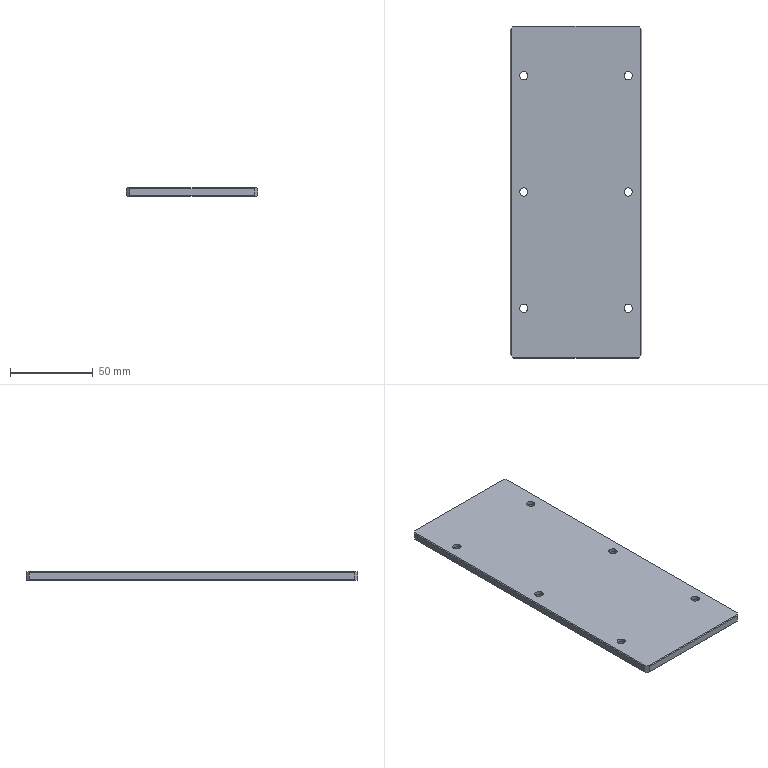Part | NX | 1 solid | 48 faces | box 79 x 200 x 5 mm | volume 77567 mm3 | plane 24 | cylinder 24 | commonest cylinder face diameters 5 x12 8.5 x12
STEP:
#1=CARTESIAN_POINT('',(1.5,199.5,1.5));
#2=VERTEX_POINT('',#1);
#3=CARTESIAN_POINT('',(77.5,199.5,1.5));
#4=VERTEX_POINT('',#3);
#5=CARTESIAN_POINT('',(0.,199.5,1.5));
#6=DIRECTION('',(1.,0.,0.));
#7=VECTOR('',#6,1000.);
#8=LINE('',#5,#7);
#9=EDGE_CURVE('',#2,#4,#8,.T.);
#10=ORIENTED_EDGE('',*,*,#9,.F.);
#11=CARTESIAN_POINT('',(0.5,198.5,1.5));
#12=VERTEX_POINT('',#11);
#13=CARTESIAN_POINT('',(-198.,0.,1.5));
#14=DIRECTION('',(-0.7071,-0.7071,0.));
#15=VECTOR('',#14,1000.);
#16=LINE('',#13,#15);
#17=EDGE_CURVE('',#2,#12,#16,.T.);
#18=ORIENTED_EDGE('',*,*,#17,.T.);
#19=CARTESIAN_POINT('',(0.5,1.5,1.5));
#20=VERTEX_POINT('',#19);
#21=CARTESIAN_POINT('',(0.5,0.,1.5));
#22=DIRECTION('',(0.,1.,0.));
#23=VECTOR('',#22,1000.);
#24=LINE('',#21,#23);
#25=EDGE_CURVE('',#20,#12,#24,.T.);
#26=ORIENTED_EDGE('',*,*,#25,.F.);
#27=CARTESIAN_POINT('',(1.5,0.5,1.5));
#28=VERTEX_POINT('',#27);
#29=CARTESIAN_POINT('',(2.,0.,1.5));
#30=DIRECTION('',(0.7071,-0.7071,0.));
#31=VECTOR('',#30,1000.);
#32=LINE('',#29,#31);
#33=EDGE_CURVE('',#20,#28,#32,.T.);
#34=ORIENTED_EDGE('',*,*,#33,.T.);
#35=CARTESIAN_POINT('',(77.5,0.5,1.5));
#36=VERTEX_POINT('',#35);
#37=CARTESIAN_POINT('',(0.,0.5,1.5));
#38=DIRECTION('',(-1.,0.,0.));
#39=VECTOR('',#38,1000.);
#40=LINE('',#37,#39);
#41=EDGE_CURVE('',#36,#28,#40,.T.);
#42=ORIENTED_EDGE('',*,*,#41,.F.);
#43=CARTESIAN_POINT('',(78.5,1.5,1.5));
#44=VERTEX_POINT('',#43);
#45=CARTESIAN_POINT('',(77.,0.,1.5));
#46=DIRECTION('',(-0.7071,-0.7071,0.));
#47=VECTOR('',#46,1000.);
#48=LINE('',#45,#47);
#49=EDGE_CURVE('',#44,#36,#48,.T.);
#50=ORIENTED_EDGE('',*,*,#49,.F.);
#51=CARTESIAN_POINT('',(78.5,198.5,1.5));
#52=VERTEX_POINT('',#51);
#53=CARTESIAN_POINT('',(78.5,0.,1.5));
#54=DIRECTION('',(0.,-1.,0.));
#55=VECTOR('',#54,1000.);
#56=LINE('',#53,#55);
#57=EDGE_CURVE('',#52,#44,#56,.T.);
#58=ORIENTED_EDGE('',*,*,#57,.F.);
#59=CARTESIAN_POINT('',(277.,0.,1.5));
#60=DIRECTION('',(0.7071,-0.7071,0.));
#61=VECTOR('',#60,1000.);
#62=LINE('',#59,#61);
#63=EDGE_CURVE('',#4,#52,#62,.T.);
#64=ORIENTED_EDGE('',*,*,#63,.F.);
#65=EDGE_LOOP('',(#10,#18,#26,#34,#42,#50,#58,#64));
#66=FACE_BOUND('',#65,.T.);
#67=CARTESIAN_POINT('',(68.5,30.,1.5));
#68=VERTEX_POINT('',#67);
#69=CARTESIAN_POINT('',(73.5,30.,1.5));
#70=VERTEX_POINT('',#69);
#71=CARTESIAN_POINT('',(71.,30.,1.5));
#72=DIRECTION('',(0.,0.,1.));
#73=DIRECTION('',(1.,0.,0.));
#74=AXIS2_PLACEMENT_3D('',#71,#72,#73);
#75=CIRCLE('',#74,2.5);
#76=EDGE_CURVE('',#68,#70,#75,.T.);
#77=ORIENTED_EDGE('',*,*,#76,.F.);
#78=CARTESIAN_POINT('',(71.,30.,1.5));
#79=DIRECTION('',(0.,0.,1.));
#80=DIRECTION('',(1.,0.,0.));
#81=AXIS2_PLACEMENT_3D('',#78,#79,#80);
#82=CIRCLE('',#81,2.5);
#83=EDGE_CURVE('',#70,#68,#82,.T.);
#84=ORIENTED_EDGE('',*,*,#83,.F.);
#85=EDGE_LOOP('',(#77,#84));
#86=FACE_BOUND('',#85,.T.);
#87=CARTESIAN_POINT('',(68.5,100.,1.5));
#88=VERTEX_POINT('',#87);
#89=CARTESIAN_POINT('',(73.5,100.,1.5));
#90=VERTEX_POINT('',#89);
#91=CARTESIAN_POINT('',(71.,100.,1.5));
#92=DIRECTION('',(0.,0.,1.));
#93=DIRECTION('',(1.,0.,0.));
#94=AXIS2_PLACEMENT_3D('',#91,#92,#93);
#95=CIRCLE('',#94,2.5);
#96=EDGE_CURVE('',#88,#90,#95,.T.);
#97=ORIENTED_EDGE('',*,*,#96,.F.);
#98=CARTESIAN_POINT('',(71.,100.,1.5));
#99=DIRECTION('',(0.,0.,1.));
#100=DIRECTION('',(1.,0.,0.));
#101=AXIS2_PLACEMENT_3D('',#98,#99,#100);
#102=CIRCLE('',#101,2.5);
#103=EDGE_CURVE('',#90,#88,#102,.T.);
#104=ORIENTED_EDGE('',*,*,#103,.F.);
#105=EDGE_LOOP('',(#97,#104));
#106=FACE_BOUND('',#105,.T.);
#107=CARTESIAN_POINT('',(73.5,170.,1.5));
#108=VERTEX_POINT('',#107);
#109=CARTESIAN_POINT('',(68.5,170.,1.5));
#110=VERTEX_POINT('',#109);
#111=CARTESIAN_POINT('',(71.,170.,1.5));
#112=DIRECTION('',(0.,0.,1.));
#113=DIRECTION('',(1.,0.,0.));
#114=AXIS2_PLACEMENT_3D('',#111,#112,#113);
#115=CIRCLE('',#114,2.5);
#116=EDGE_CURVE('',#108,#110,#115,.T.);
#117=ORIENTED_EDGE('',*,*,#116,.F.);
#118=CARTESIAN_POINT('',(71.,170.,1.5));
#119=DIRECTION('',(0.,0.,1.));
#120=DIRECTION('',(1.,0.,0.));
#121=AXIS2_PLACEMENT_3D('',#118,#119,#120);
#122=CIRCLE('',#121,2.5);
#123=EDGE_CURVE('',#110,#108,#122,.T.);
#124=ORIENTED_EDGE('',*,*,#123,.F.);
#125=EDGE_LOOP('',(#117,#124));
#126=FACE_BOUND('',#125,.T.);
#127=CARTESIAN_POINT('',(10.5,30.,1.5));
#128=VERTEX_POINT('',#127);
#129=CARTESIAN_POINT('',(5.5,30.,1.5));
#130=VERTEX_POINT('',#129);
#131=CARTESIAN_POINT('',(8.,30.,1.5));
#132=DIRECTION('',(0.,0.,1.));
#133=DIRECTION('',(1.,0.,0.));
#134=AXIS2_PLACEMENT_3D('',#131,#132,#133);
#135=CIRCLE('',#134,2.5);
#136=EDGE_CURVE('',#128,#130,#135,.T.);
#137=ORIENTED_EDGE('',*,*,#136,.F.);
#138=CARTESIAN_POINT('',(8.,30.,1.5));
#139=DIRECTION('',(0.,0.,1.));
#140=DIRECTION('',(1.,0.,0.));
#141=AXIS2_PLACEMENT_3D('',#138,#139,#140);
#142=CIRCLE('',#141,2.5);
#143=EDGE_CURVE('',#130,#128,#142,.T.);
#144=ORIENTED_EDGE('',*,*,#143,.F.);
#145=EDGE_LOOP('',(#137,#144));
#146=FACE_BOUND('',#145,.T.);
#147=CARTESIAN_POINT('',(5.5,100.,1.5));
#148=VERTEX_POINT('',#147);
#149=CARTESIAN_POINT('',(10.5,100.,1.5));
#150=VERTEX_POINT('',#149);
#151=CARTESIAN_POINT('',(8.,100.,1.5));
#152=DIRECTION('',(0.,0.,1.));
#153=DIRECTION('',(1.,0.,0.));
#154=AXIS2_PLACEMENT_3D('',#151,#152,#153);
#155=CIRCLE('',#154,2.5);
#156=EDGE_CURVE('',#148,#150,#155,.T.);
#157=ORIENTED_EDGE('',*,*,#156,.F.);
#158=CARTESIAN_POINT('',(8.,100.,1.5));
#159=DIRECTION('',(0.,0.,1.));
#160=DIRECTION('',(1.,0.,0.));
#161=AXIS2_PLACEMENT_3D('',#158,#159,#160);
#162=CIRCLE('',#161,2.5);
#163=EDGE_CURVE('',#150,#148,#162,.T.);
#164=ORIENTED_EDGE('',*,*,#163,.F.);
#165=EDGE_LOOP('',(#157,#164));
#166=FACE_BOUND('',#165,.T.);
#167=CARTESIAN_POINT('',(10.5,170.,1.5));
#168=VERTEX_POINT('',#167);
#169=CARTESIAN_POINT('',(5.5,170.,1.5));
#170=VERTEX_POINT('',#169);
#171=CARTESIAN_POINT('',(8.,170.,1.5));
#172=DIRECTION('',(0.,0.,1.));
#173=DIRECTION('',(1.,0.,0.));
#174=AXIS2_PLACEMENT_3D('',#171,#172,#173);
#175=CIRCLE('',#174,2.5);
#176=EDGE_CURVE('',#168,#170,#175,.T.);
#177=ORIENTED_EDGE('',*,*,#176,.F.);
#178=CARTESIAN_POINT('',(8.,170.,1.5));
#179=DIRECTION('',(0.,0.,1.));
#180=DIRECTION('',(1.,0.,0.));
#181=AXIS2_PLACEMENT_3D('',#178,#179,#180);
#182=CIRCLE('',#181,2.5);
#183=EDGE_CURVE('',#170,#168,#182,.T.);
#184=ORIENTED_EDGE('',*,*,#183,.F.);
#185=EDGE_LOOP('',(#177,#184));
#186=FACE_BOUND('',#185,.T.);
#187=CARTESIAN_POINT('',(0.,0.,1.5));
#188=DIRECTION('',(0.,0.,1.));
#189=DIRECTION('',(1.,0.,0.));
#190=AXIS2_PLACEMENT_3D('',#187,#188,#189);
#191=PLANE('',#190);
#192=ADVANCED_FACE('',(#66,#86,#106,#126,#146,#166,#186),#191,.T.);
#193=CARTESIAN_POINT('',(12.25,100.,-0.5));
#194=VERTEX_POINT('',#193);
#195=CARTESIAN_POINT('',(3.75,100.,-0.5));
#196=VERTEX_POINT('',#195);
#197=CARTESIAN_POINT('',(8.,100.,-0.5));
#198=DIRECTION('',(0.,0.,-1.));
#199=DIRECTION('',(1.,0.,0.));
#200=AXIS2_PLACEMENT_3D('',#197,#198,#199);
#201=CIRCLE('',#200,4.25);
#202=EDGE_CURVE('',#194,#196,#201,.T.);
#203=ORIENTED_EDGE('',*,*,#202,.T.);
#204=CARTESIAN_POINT('',(8.,100.,-0.5));
#205=DIRECTION('',(0.,0.,-1.));
#206=DIRECTION('',(1.,0.,0.));
#207=AXIS2_PLACEMENT_3D('',#204,#205,#206);
#208=CIRCLE('',#207,4.25);
#209=EDGE_CURVE('',#196,#194,#208,.T.);
#210=ORIENTED_EDGE('',*,*,#209,.T.);
#211=EDGE_LOOP('',(#203,#210));
#212=FACE_BOUND('',#211,.T.);
#213=CARTESIAN_POINT('',(10.5,100.,-0.5));
#214=VERTEX_POINT('',#213);
#215=CARTESIAN_POINT('',(5.5,100.,-0.5));
#216=VERTEX_POINT('',#215);
#217=CARTESIAN_POINT('',(8.,100.,-0.5));
#218=DIRECTION('',(0.,0.,1.));
#219=DIRECTION('',(1.,0.,0.));
#220=AXIS2_PLACEMENT_3D('',#217,#218,#219);
#221=CIRCLE('',#220,2.5);
#222=EDGE_CURVE('',#214,#216,#221,.T.);
#223=ORIENTED_EDGE('',*,*,#222,.T.);
#224=CARTESIAN_POINT('',(8.,100.,-0.5));
#225=DIRECTION('',(0.,0.,1.));
#226=DIRECTION('',(1.,0.,0.));
#227=AXIS2_PLACEMENT_3D('',#224,#225,#226);
#228=CIRCLE('',#227,2.5);
#229=EDGE_CURVE('',#216,#214,#228,.T.);
#230=ORIENTED_EDGE('',*,*,#229,.T.);
#231=EDGE_LOOP('',(#223,#230));
#232=FACE_BOUND('',#231,.T.);
#233=CARTESIAN_POINT('',(28.959,9.742,-0.5));
#234=DIRECTION('',(0.,0.,-1.));
#235=DIRECTION('',(0.,-1.,0.));
#236=AXIS2_PLACEMENT_3D('',#233,#234,#235);
#237=PLANE('',#236);
#238=ADVANCED_FACE('',(#212,#232),#237,.T.);
#239=CARTESIAN_POINT('',(2.,0.,1.));
#240=VERTEX_POINT('',#239);
#241=CARTESIAN_POINT('',(77.,0.,1.));
#242=VERTEX_POINT('',#241);
#243=CARTESIAN_POINT('',(0.,0.,1.));
#244=DIRECTION('',(1.,0.,0.));
#245=VECTOR('',#244,1000.);
#246=LINE('',#243,#245);
#247=EDGE_CURVE('',#240,#242,#246,.T.);
#248=ORIENTED_EDGE('',*,*,#247,.F.);
#249=CARTESIAN_POINT('',(2.,0.,-3.));
#250=VERTEX_POINT('',#249);
#251=CARTESIAN_POINT('',(2.,0.,0.));
#252=DIRECTION('',(0.,0.,-1.));
#253=VECTOR('',#252,1000.);
#254=LINE('',#251,#253);
#255=EDGE_CURVE('',#240,#250,#254,.T.);
#256=ORIENTED_EDGE('',*,*,#255,.T.);
#257=CARTESIAN_POINT('',(77.,0.,-3.));
#258=VERTEX_POINT('',#257);
#259=CARTESIAN_POINT('',(0.,0.,-3.));
#260=DIRECTION('',(-1.,0.,0.));
#261=VECTOR('',#260,1000.);
#262=LINE('',#259,#261);
#263=EDGE_CURVE('',#258,#250,#262,.T.);
#264=ORIENTED_EDGE('',*,*,#263,.F.);
#265=CARTESIAN_POINT('',(77.,0.,0.));
#266=DIRECTION('',(0.,0.,-1.));
#267=VECTOR('',#266,1000.);
#268=LINE('',#265,#267);
#269=EDGE_CURVE('',#242,#258,#268,.T.);
#270=ORIENTED_EDGE('',*,*,#269,.F.);
#271=EDGE_LOOP('',(#248,#256,#264,#270));
#272=FACE_BOUND('',#271,.T.);
#273=CARTESIAN_POINT('',(0.,0.,0.));
#274=DIRECTION('',(0.,-1.,0.));
#275=DIRECTION('',(0.,0.,-1.));
#276=AXIS2_PLACEMENT_3D('',#273,#274,#275);
#277=PLANE('',#276);
#278=ADVANCED_FACE('',(#272),#277,.T.);
#279=ORIENTED_EDGE('',*,*,#202,.F.);
#280=CARTESIAN_POINT('',(12.25,100.,-3.5));
#281=VERTEX_POINT('',#280);
#282=CARTESIAN_POINT('',(12.25,100.,-3.5));
#283=DIRECTION('',(0.,0.,-1.));
#284=VECTOR('',#283,1000.);
#285=LINE('',#282,#284);
#286=EDGE_CURVE('',#194,#281,#285,.T.);
#287=ORIENTED_EDGE('',*,*,#286,.T.);
#288=CARTESIAN_POINT('',(3.75,100.,-3.5));
#289=VERTEX_POINT('',#288);
#290=CARTESIAN_POINT('',(8.,100.,-3.5));
#291=DIRECTION('',(0.,0.,-1.));
#292=DIRECTION('',(1.,0.,0.));
#293=AXIS2_PLACEMENT_3D('',#290,#291,#292);
#294=CIRCLE('',#293,4.25);
#295=EDGE_CURVE('',#281,#289,#294,.T.);
#296=ORIENTED_EDGE('',*,*,#295,.T.);
#297=CARTESIAN_POINT('',(3.75,100.,-3.5));
#298=DIRECTION('',(0.,0.,-1.));
#299=VECTOR('',#298,1000.);
#300=LINE('',#297,#299);
#301=EDGE_CURVE('',#196,#289,#300,.T.);
#302=ORIENTED_EDGE('',*,*,#301,.F.);
#303=EDGE_LOOP('',(#279,#287,#296,#302));
#304=FACE_BOUND('',#303,.T.);
#305=CARTESIAN_POINT('',(8.,100.,-3.5));
#306=DIRECTION('',(0.,0.,-1.));
#307=DIRECTION('',(1.,0.,0.));
#308=AXIS2_PLACEMENT_3D('',#305,#306,#307);
#309=CYLINDRICAL_SURFACE('',#308,4.25);
#310=ADVANCED_FACE('',(#304),#309,.F.);
#311=CARTESIAN_POINT('',(0.,198.,1.));
#312=VERTEX_POINT('',#311);
#313=CARTESIAN_POINT('',(0.,2.,1.));
#314=VERTEX_POINT('',#313);
#315=CARTESIAN_POINT('',(0.,0.,1.));
#316=DIRECTION('',(0.,-1.,0.));
#317=VECTOR('',#316,1000.);
#318=LINE('',#315,#317);
#319=EDGE_CURVE('',#312,#314,#318,.T.);
#320=ORIENTED_EDGE('',*,*,#319,.F.);
#321=CARTESIAN_POINT('',(0.,198.,-3.));
#322=VERTEX_POINT('',#321);
#323=CARTESIAN_POINT('',(0.,198.,0.));
#324=DIRECTION('',(0.,0.,-1.));
#325=VECTOR('',#324,1000.);
#326=LINE('',#323,#325);
#327=EDGE_CURVE('',#312,#322,#326,.T.);
#328=ORIENTED_EDGE('',*,*,#327,.T.);
#329=CARTESIAN_POINT('',(0.,2.,-3.));
#330=VERTEX_POINT('',#329);
#331=CARTESIAN_POINT('',(0.,0.,-3.));
#332=DIRECTION('',(0.,1.,0.));
#333=VECTOR('',#332,1000.);
#334=LINE('',#331,#333);
#335=EDGE_CURVE('',#330,#322,#334,.T.);
#336=ORIENTED_EDGE('',*,*,#335,.F.);
#337=CARTESIAN_POINT('',(0.,2.,0.));
#338=DIRECTION('',(0.,0.,1.));
#339=VECTOR('',#338,1000.);
#340=LINE('',#337,#339);
#341=EDGE_CURVE('',#330,#314,#340,.T.);
#342=ORIENTED_EDGE('',*,*,#341,.T.);
#343=EDGE_LOOP('',(#320,#328,#336,#342));
#344=FACE_BOUND('',#343,.T.);
#345=CARTESIAN_POINT('',(0.,200.,0.));
#346=DIRECTION('',(-1.,0.,0.));
#347=DIRECTION('',(0.,0.,1.));
#348=AXIS2_PLACEMENT_3D('',#345,#346,#347);
#349=PLANE('',#348);
#350=ADVANCED_FACE('',(#344),#349,.T.);
#351=CARTESIAN_POINT('',(3.75,170.,-0.5));
#352=VERTEX_POINT('',#351);
#353=CARTESIAN_POINT('',(12.25,170.,-0.5));
#354=VERTEX_POINT('',#353);
#355=CARTESIAN_POINT('',(8.,170.,-0.5));
#356=DIRECTION('',(0.,0.,-1.));
#357=DIRECTION('',(1.,0.,0.));
#358=AXIS2_PLACEMENT_3D('',#355,#356,#357);
#359=CIRCLE('',#358,4.25);
#360=EDGE_CURVE('',#352,#354,#359,.T.);
#361=ORIENTED_EDGE('',*,*,#360,.T.);
#362=CARTESIAN_POINT('',(8.,170.,-0.5));
#363=DIRECTION('',(0.,0.,-1.));
#364=DIRECTION('',(1.,0.,0.));
#365=AXIS2_PLACEMENT_3D('',#362,#363,#364);
#366=CIRCLE('',#365,4.25);
#367=EDGE_CURVE('',#354,#352,#366,.T.);
#368=ORIENTED_EDGE('',*,*,#367,.T.);
#369=EDGE_LOOP('',(#361,#368));
#370=FACE_BOUND('',#369,.T.);
#371=CARTESIAN_POINT('',(10.5,170.,-0.5));
#372=VERTEX_POINT('',#371);
#373=CARTESIAN_POINT('',(5.5,170.,-0.5));
#374=VERTEX_POINT('',#373);
#375=CARTESIAN_POINT('',(8.,170.,-0.5));
#376=DIRECTION('',(0.,0.,1.));
#377=DIRECTION('',(1.,0.,0.));
#378=AXIS2_PLACEMENT_3D('',#375,#376,#377);
#379=CIRCLE('',#378,2.5);
#380=EDGE_CURVE('',#372,#374,#379,.T.);
#381=ORIENTED_EDGE('',*,*,#380,.T.);
#382=CARTESIAN_POINT('',(8.,170.,-0.5));
#383=DIRECTION('',(0.,0.,1.));
#384=DIRECTION('',(1.,0.,0.));
#385=AXIS2_PLACEMENT_3D('',#382,#383,#384);
#386=CIRCLE('',#385,2.5);
#387=EDGE_CURVE('',#374,#372,#386,.T.);
#388=ORIENTED_EDGE('',*,*,#387,.T.);
#389=EDGE_LOOP('',(#381,#388));
#390=FACE_BOUND('',#389,.T.);
#391=CARTESIAN_POINT('',(28.959,9.742,-0.5));
#392=DIRECTION('',(0.,0.,-1.));
#393=DIRECTION('',(0.,-1.,0.));
#394=AXIS2_PLACEMENT_3D('',#391,#392,#393);
#395=PLANE('',#394);
#396=ADVANCED_FACE('',(#370,#390),#395,.T.);
#397=CARTESIAN_POINT('',(77.,200.,1.));
#398=VERTEX_POINT('',#397);
#399=CARTESIAN_POINT('',(2.,200.,1.));
#400=VERTEX_POINT('',#399);
#401=CARTESIAN_POINT('',(0.,200.,1.));
#402=DIRECTION('',(-1.,0.,0.));
#403=VECTOR('',#402,1000.);
#404=LINE('',#401,#403);
#405=EDGE_CURVE('',#398,#400,#404,.T.);
#406=ORIENTED_EDGE('',*,*,#405,.F.);
#407=CARTESIAN_POINT('',(77.,200.,-3.));
#408=VERTEX_POINT('',#407);
#409=CARTESIAN_POINT('',(77.,200.,0.));
#410=DIRECTION('',(0.,0.,1.));
#411=VECTOR('',#410,1000.);
#412=LINE('',#409,#411);
#413=EDGE_CURVE('',#408,#398,#412,.T.);
#414=ORIENTED_EDGE('',*,*,#413,.F.);
#415=CARTESIAN_POINT('',(2.,200.,-3.));
#416=VERTEX_POINT('',#415);
#417=CARTESIAN_POINT('',(0.,200.,-3.));
#418=DIRECTION('',(1.,0.,0.));
#419=VECTOR('',#418,1000.);
#420=LINE('',#417,#419);
#421=EDGE_CURVE('',#416,#408,#420,.T.);
#422=ORIENTED_EDGE('',*,*,#421,.F.);
#423=CARTESIAN_POINT('',(2.,200.,0.));
#424=DIRECTION('',(0.,0.,1.));
#425=VECTOR('',#424,1000.);
#426=LINE('',#423,#425);
#427=EDGE_CURVE('',#416,#400,#426,.T.);
#428=ORIENTED_EDGE('',*,*,#427,.T.);
#429=EDGE_LOOP('',(#406,#414,#422,#428));
#430=FACE_BOUND('',#429,.T.);
#431=CARTESIAN_POINT('',(79.,200.,0.));
#432=DIRECTION('',(0.,1.,0.));
#433=DIRECTION('',(1.,0.,0.));
#434=AXIS2_PLACEMENT_3D('',#431,#432,#433);
#435=PLANE('',#434);
#436=ADVANCED_FACE('',(#430),#435,.T.);
#437=CARTESIAN_POINT('',(12.25,170.,-3.5));
#438=VERTEX_POINT('',#437);
#439=CARTESIAN_POINT('',(3.75,170.,-3.5));
#440=VERTEX_POINT('',#439);
#441=CARTESIAN_POINT('',(8.,170.,-3.5));
#442=DIRECTION('',(0.,0.,-1.));
#443=DIRECTION('',(1.,0.,0.));
#444=AXIS2_PLACEMENT_3D('',#441,#442,#443);
#445=CIRCLE('',#444,4.25);
#446=EDGE_CURVE('',#438,#440,#445,.T.);
#447=ORIENTED_EDGE('',*,*,#446,.T.);
#448=CARTESIAN_POINT('',(3.75,170.,-3.5));
#449=DIRECTION('',(0.,0.,-1.));
#450=VECTOR('',#449,1000.);
#451=LINE('',#448,#450);
#452=EDGE_CURVE('',#440,#352,#451,.F.);
#453=ORIENTED_EDGE('',*,*,#452,.T.);
#454=ORIENTED_EDGE('',*,*,#367,.F.);
#455=CARTESIAN_POINT('',(12.25,170.,-3.5));
#456=DIRECTION('',(0.,0.,-1.));
#457=VECTOR('',#456,1000.);
#458=LINE('',#455,#457);
#459=EDGE_CURVE('',#438,#354,#458,.F.);
#460=ORIENTED_EDGE('',*,*,#459,.F.);
#461=EDGE_LOOP('',(#447,#453,#454,#460));
#462=FACE_BOUND('',#461,.T.);
#463=CARTESIAN_POINT('',(8.,170.,-3.5));
#464=DIRECTION('',(0.,0.,-1.));
#465=DIRECTION('',(1.,0.,0.));
#466=AXIS2_PLACEMENT_3D('',#463,#464,#465);
#467=CYLINDRICAL_SURFACE('',#466,4.25);
#468=ADVANCED_FACE('',(#462),#467,.F.);
#469=CARTESIAN_POINT('',(79.,2.,1.));
#470=VERTEX_POINT('',#469);
#471=CARTESIAN_POINT('',(79.,198.,1.));
#472=VERTEX_POINT('',#471);
#473=CARTESIAN_POINT('',(79.,0.,1.));
#474=DIRECTION('',(0.,1.,0.));
#475=VECTOR('',#474,1000.);
#476=LINE('',#473,#475);
#477=EDGE_CURVE('',#470,#472,#476,.T.);
#478=ORIENTED_EDGE('',*,*,#477,.F.);
#479=CARTESIAN_POINT('',(79.,2.,-3.));
#480=VERTEX_POINT('',#479);
#481=CARTESIAN_POINT('',(79.,2.,0.));
#482=DIRECTION('',(0.,0.,1.));
#483=VECTOR('',#482,1000.);
#484=LINE('',#481,#483);
#485=EDGE_CURVE('',#480,#470,#484,.T.);
#486=ORIENTED_EDGE('',*,*,#485,.F.);
#487=CARTESIAN_POINT('',(79.,198.,-3.));
#488=VERTEX_POINT('',#487);
#489=CARTESIAN_POINT('',(79.,0.,-3.));
#490=DIRECTION('',(0.,-1.,0.));
#491=VECTOR('',#490,1000.);
#492=LINE('',#489,#491);
#493=EDGE_CURVE('',#488,#480,#492,.T.);
#494=ORIENTED_EDGE('',*,*,#493,.F.);
#495=CARTESIAN_POINT('',(79.,198.,0.));
#496=DIRECTION('',(0.,0.,-1.));
#497=VECTOR('',#496,1000.);
#498=LINE('',#495,#497);
#499=EDGE_CURVE('',#472,#488,#498,.T.);
#500=ORIENTED_EDGE('',*,*,#499,.F.);
#501=EDGE_LOOP('',(#478,#486,#494,#500));
#502=FACE_BOUND('',#501,.T.);
#503=CARTESIAN_POINT('',(79.,0.,0.));
#504=DIRECTION('',(1.,0.,0.));
#505=DIRECTION('',(0.,1.,0.));
#506=AXIS2_PLACEMENT_3D('',#503,#504,#505);
#507=PLANE('',#506);
#508=ADVANCED_FACE('',(#502),#507,.T.);
#509=CARTESIAN_POINT('',(77.5,0.5,-3.5));
#510=VERTEX_POINT('',#509);
#511=CARTESIAN_POINT('',(1.5,0.5,-3.5));
#512=VERTEX_POINT('',#511);
#513=CARTESIAN_POINT('',(0.,0.5,-3.5));
#514=DIRECTION('',(-1.,0.,0.));
#515=VECTOR('',#514,1000.);
#516=LINE('',#513,#515);
#517=EDGE_CURVE('',#510,#512,#516,.T.);
#518=ORIENTED_EDGE('',*,*,#517,.T.);
#519=CARTESIAN_POINT('',(0.5,1.5,-3.5));
#520=VERTEX_POINT('',#519);
#521=CARTESIAN_POINT('',(2.,0.,-3.5));
#522=DIRECTION('',(0.7071,-0.7071,0.));
#523=VECTOR('',#522,1000.);
#524=LINE('',#521,#523);
#525=EDGE_CURVE('',#520,#512,#524,.T.);
#526=ORIENTED_EDGE('',*,*,#525,.F.);
#527=CARTESIAN_POINT('',(0.5,198.5,-3.5));
#528=VERTEX_POINT('',#527);
#529=CARTESIAN_POINT('',(0.5,0.,-3.5));
#530=DIRECTION('',(0.,1.,0.));
#531=VECTOR('',#530,1000.);
#532=LINE('',#529,#531);
#533=EDGE_CURVE('',#520,#528,#532,.T.);
#534=ORIENTED_EDGE('',*,*,#533,.T.);
#535=CARTESIAN_POINT('',(1.5,199.5,-3.5));
#536=VERTEX_POINT('',#535);
#537=CARTESIAN_POINT('',(-198.,0.,-3.5));
#538=DIRECTION('',(-0.7071,-0.7071,0.));
#539=VECTOR('',#538,1000.);
#540=LINE('',#537,#539);
#541=EDGE_CURVE('',#536,#528,#540,.T.);
#542=ORIENTED_EDGE('',*,*,#541,.F.);
#543=CARTESIAN_POINT('',(77.5,199.5,-3.5));
#544=VERTEX_POINT('',#543);
#545=CARTESIAN_POINT('',(0.,199.5,-3.5));
#546=DIRECTION('',(1.,0.,0.));
#547=VECTOR('',#546,1000.);
#548=LINE('',#545,#547);
#549=EDGE_CURVE('',#536,#544,#548,.T.);
#550=ORIENTED_EDGE('',*,*,#549,.T.);
#551=CARTESIAN_POINT('',(78.5,198.5,-3.5));
#552=VERTEX_POINT('',#551);
#553=CARTESIAN_POINT('',(277.,0.,-3.5));
#554=DIRECTION('',(0.7071,-0.7071,0.));
#555=VECTOR('',#554,1000.);
#556=LINE('',#553,#555);
#557=EDGE_CURVE('',#544,#552,#556,.T.);
#558=ORIENTED_EDGE('',*,*,#557,.T.);
#559=CARTESIAN_POINT('',(78.5,1.5,-3.5));
#560=VERTEX_POINT('',#559);
#561=CARTESIAN_POINT('',(78.5,0.,-3.5));
#562=DIRECTION('',(0.,-1.,0.));
#563=VECTOR('',#562,1000.);
#564=LINE('',#561,#563);
#565=EDGE_CURVE('',#552,#560,#564,.T.);
#566=ORIENTED_EDGE('',*,*,#565,.T.);
#567=CARTESIAN_POINT('',(77.,0.,-3.5));
#568=DIRECTION('',(-0.7071,-0.7071,0.));
#569=VECTOR('',#568,1000.);
#570=LINE('',#567,#569);
#571=EDGE_CURVE('',#560,#510,#570,.T.);
#572=ORIENTED_EDGE('',*,*,#571,.T.);
#573=EDGE_LOOP('',(#518,#526,#534,#542,#550,#558,#566,#572));
#574=FACE_BOUND('',#573,.T.);
#575=CARTESIAN_POINT('',(12.25,30.,-3.5));
#576=VERTEX_POINT('',#575);
#577=CARTESIAN_POINT('',(3.75,30.,-3.5));
#578=VERTEX_POINT('',#577);
#579=CARTESIAN_POINT('',(8.,30.,-3.5));
#580=DIRECTION('',(0.,0.,-1.));
#581=DIRECTION('',(1.,0.,0.));
#582=AXIS2_PLACEMENT_3D('',#579,#580,#581);
#583=CIRCLE('',#582,4.25);
#584=EDGE_CURVE('',#576,#578,#583,.T.);
#585=ORIENTED_EDGE('',*,*,#584,.F.);
#586=CARTESIAN_POINT('',(8.,30.,-3.5));
#587=DIRECTION('',(0.,0.,-1.));
#588=DIRECTION('',(1.,0.,0.));
#589=AXIS2_PLACEMENT_3D('',#586,#587,#588);
#590=CIRCLE('',#589,4.25);
#591=EDGE_CURVE('',#578,#576,#590,.T.);
#592=ORIENTED_EDGE('',*,*,#591,.F.);
#593=EDGE_LOOP('',(#585,#592));
#594=FACE_BOUND('',#593,.T.);
#595=CARTESIAN_POINT('',(66.75,170.,-3.5));
#596=VERTEX_POINT('',#595);
#597=CARTESIAN_POINT('',(75.25,170.,-3.5));
#598=VERTEX_POINT('',#597);
#599=CARTESIAN_POINT('',(71.,170.,-3.5));
#600=DIRECTION('',(0.,0.,-1.));
#601=DIRECTION('',(1.,0.,0.));
#602=AXIS2_PLACEMENT_3D('',#599,#600,#601);
#603=CIRCLE('',#602,4.25);
#604=EDGE_CURVE('',#596,#598,#603,.T.);
#605=ORIENTED_EDGE('',*,*,#604,.F.);
#606=CARTESIAN_POINT('',(71.,170.,-3.5));
#607=DIRECTION('',(0.,0.,-1.));
#608=DIRECTION('',(1.,0.,0.));
#609=AXIS2_PLACEMENT_3D('',#606,#607,#608);
#610=CIRCLE('',#609,4.25);
#611=EDGE_CURVE('',#598,#596,#610,.T.);
#612=ORIENTED_EDGE('',*,*,#611,.F.);
#613=EDGE_LOOP('',(#605,#612));
#614=FACE_BOUND('',#613,.T.);
#615=CARTESIAN_POINT('',(66.75,100.,-3.5));
#616=VERTEX_POINT('',#615);
#617=CARTESIAN_POINT('',(75.25,100.,-3.5));
#618=VERTEX_POINT('',#617);
#619=CARTESIAN_POINT('',(71.,100.,-3.5));
#620=DIRECTION('',(0.,0.,-1.));
#621=DIRECTION('',(1.,0.,0.));
#622=AXIS2_PLACEMENT_3D('',#619,#620,#621);
#623=CIRCLE('',#622,4.25);
#624=EDGE_CURVE('',#616,#618,#623,.T.);
#625=ORIENTED_EDGE('',*,*,#624,.F.);
#626=CARTESIAN_POINT('',(71.,100.,-3.5));
#627=DIRECTION('',(0.,0.,-1.));
#628=DIRECTION('',(1.,0.,0.));
#629=AXIS2_PLACEMENT_3D('',#626,#627,#628);
#630=CIRCLE('',#629,4.25);
#631=EDGE_CURVE('',#618,#616,#630,.T.);
#632=ORIENTED_EDGE('',*,*,#631,.F.);
#633=EDGE_LOOP('',(#625,#632));
#634=FACE_BOUND('',#633,.T.);
#635=CARTESIAN_POINT('',(75.25,30.,-3.5));
#636=VERTEX_POINT('',#635);
#637=CARTESIAN_POINT('',(66.75,30.,-3.5));
#638=VERTEX_POINT('',#637);
#639=CARTESIAN_POINT('',(71.,30.,-3.5));
#640=DIRECTION('',(0.,0.,-1.));
#641=DIRECTION('',(1.,0.,0.));
#642=AXIS2_PLACEMENT_3D('',#639,#640,#641);
#643=CIRCLE('',#642,4.25);
#644=EDGE_CURVE('',#636,#638,#643,.T.);
#645=ORIENTED_EDGE('',*,*,#644,.F.);
#646=CARTESIAN_POINT('',(71.,30.,-3.5));
#647=DIRECTION('',(0.,0.,-1.));
#648=DIRECTION('',(1.,0.,0.));
#649=AXIS2_PLACEMENT_3D('',#646,#647,#648);
#650=CIRCLE('',#649,4.25);
#651=EDGE_CURVE('',#638,#636,#650,.T.);
#652=ORIENTED_EDGE('',*,*,#651,.F.);
#653=EDGE_LOOP('',(#645,#652));
#654=FACE_BOUND('',#653,.T.);
#655=ORIENTED_EDGE('',*,*,#446,.F.);
#656=CARTESIAN_POINT('',(8.,170.,-3.5));
#657=DIRECTION('',(0.,0.,-1.));
#658=DIRECTION('',(1.,0.,0.));
#659=AXIS2_PLACEMENT_3D('',#656,#657,#658);
#660=CIRCLE('',#659,4.25);
#661=EDGE_CURVE('',#440,#438,#660,.T.);
#662=ORIENTED_EDGE('',*,*,#661,.F.);
#663=EDGE_LOOP('',(#655,#662));
#664=FACE_BOUND('',#663,.T.);
#665=ORIENTED_EDGE('',*,*,#295,.F.);
#666=CARTESIAN_POINT('',(8.,100.,-3.5));
#667=DIRECTION('',(0.,0.,-1.));
#668=DIRECTION('',(1.,0.,0.));
#669=AXIS2_PLACEMENT_3D('',#666,#667,#668);
#670=CIRCLE('',#669,4.25);
#671=EDGE_CURVE('',#289,#281,#670,.T.);
#672=ORIENTED_EDGE('',*,*,#671,.F.);
#673=EDGE_LOOP('',(#665,#672));
#674=FACE_BOUND('',#673,.T.);
#675=CARTESIAN_POINT('',(0.,0.,-3.5));
#676=DIRECTION('',(0.,0.,1.));
#677=DIRECTION('',(1.,0.,0.));
#678=AXIS2_PLACEMENT_3D('',#675,#676,#677);
#679=PLANE('',#678);
#680=ADVANCED_FACE('',(#574,#594,#614,#634,#654,#664,#674),#679,.F.);
#681=CARTESIAN_POINT('',(68.5,170.,-0.5));
#682=VERTEX_POINT('',#681);
#683=CARTESIAN_POINT('',(73.5,170.,-0.5));
#684=VERTEX_POINT('',#683);
#685=CARTESIAN_POINT('',(71.,170.,-0.5));
#686=DIRECTION('',(0.,0.,1.));
#687=DIRECTION('',(1.,0.,0.));
#688=AXIS2_PLACEMENT_3D('',#685,#686,#687);
#689=CIRCLE('',#688,2.5);
#690=EDGE_CURVE('',#682,#684,#689,.T.);
#691=ORIENTED_EDGE('',*,*,#690,.F.);
#692=CARTESIAN_POINT('',(68.5,170.,0.));
#693=DIRECTION('',(0.,0.,1.));
#694=VECTOR('',#693,1000.);
#695=LINE('',#692,#694);
#696=EDGE_CURVE('',#110,#682,#695,.F.);
#697=ORIENTED_EDGE('',*,*,#696,.F.);
#698=ORIENTED_EDGE('',*,*,#123,.T.);
#699=CARTESIAN_POINT('',(73.5,170.,0.));
#700=DIRECTION('',(0.,0.,1.));
#701=VECTOR('',#700,1000.);
#702=LINE('',#699,#701);
#703=EDGE_CURVE('',#108,#684,#702,.F.);
#704=ORIENTED_EDGE('',*,*,#703,.T.);
#705=EDGE_LOOP('',(#691,#697,#698,#704));
#706=FACE_BOUND('',#705,.T.);
#707=CARTESIAN_POINT('',(71.,170.,0.));
#708=DIRECTION('',(0.,0.,1.));
#709=DIRECTION('',(1.,0.,0.));
#710=AXIS2_PLACEMENT_3D('',#707,#708,#709);
#711=CYLINDRICAL_SURFACE('',#710,2.5);
#712=ADVANCED_FACE('',(#706),#711,.F.);
#713=ORIENTED_EDGE('',*,*,#156,.T.);
#714=CARTESIAN_POINT('',(10.5,100.,0.));
#715=DIRECTION('',(0.,0.,1.));
#716=VECTOR('',#715,1000.);
#717=LINE('',#714,#716);
#718=EDGE_CURVE('',#214,#150,#717,.T.);
#719=ORIENTED_EDGE('',*,*,#718,.F.);
#720=ORIENTED_EDGE('',*,*,#229,.F.);
#721=CARTESIAN_POINT('',(5.5,100.,0.));
#722=DIRECTION('',(0.,0.,1.));
#723=VECTOR('',#722,1000.);
#724=LINE('',#721,#723);
#725=EDGE_CURVE('',#216,#148,#724,.T.);
#726=ORIENTED_EDGE('',*,*,#725,.T.);
#727=EDGE_LOOP('',(#713,#719,#720,#726));
#728=FACE_BOUND('',#727,.T.);
#729=CARTESIAN_POINT('',(8.,100.,0.));
#730=DIRECTION('',(0.,0.,1.));
#731=DIRECTION('',(1.,0.,0.));
#732=AXIS2_PLACEMENT_3D('',#729,#730,#731);
#733=CYLINDRICAL_SURFACE('',#732,2.5);
#734=ADVANCED_FACE('',(#728),#733,.F.);
#735=CARTESIAN_POINT('',(73.5,100.,-0.5));
#736=VERTEX_POINT('',#735);
#737=CARTESIAN_POINT('',(68.5,100.,-0.5));
#738=VERTEX_POINT('',#737);
#739=CARTESIAN_POINT('',(71.,100.,-0.5));
#740=DIRECTION('',(0.,0.,1.));
#741=DIRECTION('',(1.,0.,0.));
#742=AXIS2_PLACEMENT_3D('',#739,#740,#741);
#743=CIRCLE('',#742,2.5);
#744=EDGE_CURVE('',#736,#738,#743,.T.);
#745=ORIENTED_EDGE('',*,*,#744,.F.);
#746=CARTESIAN_POINT('',(73.5,100.,0.));
#747=DIRECTION('',(0.,0.,1.));
#748=VECTOR('',#747,1000.);
#749=LINE('',#746,#748);
#750=EDGE_CURVE('',#736,#90,#749,.T.);
#751=ORIENTED_EDGE('',*,*,#750,.T.);
#752=ORIENTED_EDGE('',*,*,#103,.T.);
#753=CARTESIAN_POINT('',(68.5,100.,0.));
#754=DIRECTION('',(0.,0.,1.));
#755=VECTOR('',#754,1000.);
#756=LINE('',#753,#755);
#757=EDGE_CURVE('',#738,#88,#756,.T.);
#758=ORIENTED_EDGE('',*,*,#757,.F.);
#759=EDGE_LOOP('',(#745,#751,#752,#758));
#760=FACE_BOUND('',#759,.T.);
#761=CARTESIAN_POINT('',(71.,100.,0.));
#762=DIRECTION('',(0.,0.,1.));
#763=DIRECTION('',(1.,0.,0.));
#764=AXIS2_PLACEMENT_3D('',#761,#762,#763);
#765=CYLINDRICAL_SURFACE('',#764,2.5);
#766=ADVANCED_FACE('',(#760),#765,.F.);
#767=ORIENTED_EDGE('',*,*,#380,.F.);
#768=CARTESIAN_POINT('',(10.5,170.,0.));
#769=DIRECTION('',(0.,0.,1.));
#770=VECTOR('',#769,1000.);
#771=LINE('',#768,#770);
#772=EDGE_CURVE('',#372,#168,#771,.T.);
#773=ORIENTED_EDGE('',*,*,#772,.T.);
#774=ORIENTED_EDGE('',*,*,#176,.T.);
#775=CARTESIAN_POINT('',(5.5,170.,0.));
#776=DIRECTION('',(0.,0.,1.));
#777=VECTOR('',#776,1000.);
#778=LINE('',#775,#777);
#779=EDGE_CURVE('',#374,#170,#778,.T.);
#780=ORIENTED_EDGE('',*,*,#779,.F.);
#781=EDGE_LOOP('',(#767,#773,#774,#780));
#782=FACE_BOUND('',#781,.T.);
#783=CARTESIAN_POINT('',(8.,170.,0.));
#784=DIRECTION('',(0.,0.,1.));
#785=DIRECTION('',(1.,0.,0.));
#786=AXIS2_PLACEMENT_3D('',#783,#784,#785);
#787=CYLINDRICAL_SURFACE('',#786,2.5);
#788=ADVANCED_FACE('',(#782),#787,.F.);
#789=ORIENTED_EDGE('',*,*,#76,.T.);
#790=CARTESIAN_POINT('',(73.5,30.,-0.5));
#791=VERTEX_POINT('',#790);
#792=CARTESIAN_POINT('',(73.5,30.,0.));
#793=DIRECTION('',(0.,0.,1.));
#794=VECTOR('',#793,1000.);
#795=LINE('',#792,#794);
#796=EDGE_CURVE('',#791,#70,#795,.T.);
#797=ORIENTED_EDGE('',*,*,#796,.F.);
#798=CARTESIAN_POINT('',(68.5,30.,-0.5));
#799=VERTEX_POINT('',#798);
#800=CARTESIAN_POINT('',(71.,30.,-0.5));
#801=DIRECTION('',(0.,0.,1.));
#802=DIRECTION('',(1.,0.,0.));
#803=AXIS2_PLACEMENT_3D('',#800,#801,#802);
#804=CIRCLE('',#803,2.5);
#805=EDGE_CURVE('',#799,#791,#804,.T.);
#806=ORIENTED_EDGE('',*,*,#805,.F.);
#807=CARTESIAN_POINT('',(68.5,30.,0.));
#808=DIRECTION('',(0.,0.,1.));
#809=VECTOR('',#808,1000.);
#810=LINE('',#807,#809);
#811=EDGE_CURVE('',#799,#68,#810,.T.);
#812=ORIENTED_EDGE('',*,*,#811,.T.);
#813=EDGE_LOOP('',(#789,#797,#806,#812));
#814=FACE_BOUND('',#813,.T.);
#815=CARTESIAN_POINT('',(71.,30.,0.));
#816=DIRECTION('',(0.,0.,1.));
#817=DIRECTION('',(1.,0.,0.));
#818=AXIS2_PLACEMENT_3D('',#815,#816,#817);
#819=CYLINDRICAL_SURFACE('',#818,2.5);
#820=ADVANCED_FACE('',(#814),#819,.F.);
#821=ORIENTED_EDGE('',*,*,#136,.T.);
#822=CARTESIAN_POINT('',(5.5,30.,-0.5));
#823=VERTEX_POINT('',#822);
#824=CARTESIAN_POINT('',(5.5,30.,0.));
#825=DIRECTION('',(0.,0.,1.));
#826=VECTOR('',#825,1000.);
#827=LINE('',#824,#826);
#828=EDGE_CURVE('',#823,#130,#827,.T.);
#829=ORIENTED_EDGE('',*,*,#828,.F.);
#830=CARTESIAN_POINT('',(10.5,30.,-0.5));
#831=VERTEX_POINT('',#830);
#832=CARTESIAN_POINT('',(8.,30.,-0.5));
#833=DIRECTION('',(0.,0.,1.));
#834=DIRECTION('',(1.,0.,0.));
#835=AXIS2_PLACEMENT_3D('',#832,#833,#834);
#836=CIRCLE('',#835,2.5);
#837=EDGE_CURVE('',#831,#823,#836,.T.);
#838=ORIENTED_EDGE('',*,*,#837,.F.);
#839=CARTESIAN_POINT('',(10.5,30.,0.));
#840=DIRECTION('',(0.,0.,1.));
#841=VECTOR('',#840,1000.);
#842=LINE('',#839,#841);
#843=EDGE_CURVE('',#831,#128,#842,.T.);
#844=ORIENTED_EDGE('',*,*,#843,.T.);
#845=EDGE_LOOP('',(#821,#829,#838,#844));
#846=FACE_BOUND('',#845,.T.);
#847=CARTESIAN_POINT('',(8.,30.,0.));
#848=DIRECTION('',(0.,0.,1.));
#849=DIRECTION('',(1.,0.,0.));
#850=AXIS2_PLACEMENT_3D('',#847,#848,#849);
#851=CYLINDRICAL_SURFACE('',#850,2.5);
#852=ADVANCED_FACE('',(#846),#851,.F.);
#853=CARTESIAN_POINT('',(12.25,30.,-0.5));
#854=VERTEX_POINT('',#853);
#855=CARTESIAN_POINT('',(3.75,30.,-0.5));
#856=VERTEX_POINT('',#855);
#857=CARTESIAN_POINT('',(8.,30.,-0.5));
#858=DIRECTION('',(0.,0.,-1.));
#859=DIRECTION('',(1.,0.,0.));
#860=AXIS2_PLACEMENT_3D('',#857,#858,#859);
#861=CIRCLE('',#860,4.25);
#862=EDGE_CURVE('',#854,#856,#861,.T.);
#863=ORIENTED_EDGE('',*,*,#862,.F.);
#864=CARTESIAN_POINT('',(12.25,30.,-3.5));
#865=DIRECTION('',(0.,0.,-1.));
#866=VECTOR('',#865,1000.);
#867=LINE('',#864,#866);
#868=EDGE_CURVE('',#854,#576,#867,.T.);
#869=ORIENTED_EDGE('',*,*,#868,.T.);
#870=ORIENTED_EDGE('',*,*,#584,.T.);
#871=CARTESIAN_POINT('',(3.75,30.,-3.5));
#872=DIRECTION('',(0.,0.,-1.));
#873=VECTOR('',#872,1000.);
#874=LINE('',#871,#873);
#875=EDGE_CURVE('',#856,#578,#874,.T.);
#876=ORIENTED_EDGE('',*,*,#875,.F.);
#877=EDGE_LOOP('',(#863,#869,#870,#876));
#878=FACE_BOUND('',#877,.T.);
#879=CARTESIAN_POINT('',(8.,30.,-3.5));
#880=DIRECTION('',(0.,0.,-1.));
#881=DIRECTION('',(1.,0.,0.));
#882=AXIS2_PLACEMENT_3D('',#879,#880,#881);
#883=CYLINDRICAL_SURFACE('',#882,4.25);
#884=ADVANCED_FACE('',(#878),#883,.F.);
#885=ORIENTED_EDGE('',*,*,#862,.T.);
#886=CARTESIAN_POINT('',(8.,30.,-0.5));
#887=DIRECTION('',(0.,0.,-1.));
#888=DIRECTION('',(1.,0.,0.));
#889=AXIS2_PLACEMENT_3D('',#886,#887,#888);
#890=CIRCLE('',#889,4.25);
#891=EDGE_CURVE('',#856,#854,#890,.T.);
#892=ORIENTED_EDGE('',*,*,#891,.T.);
#893=EDGE_LOOP('',(#885,#892));
#894=FACE_BOUND('',#893,.T.);
#895=ORIENTED_EDGE('',*,*,#837,.T.);
#896=CARTESIAN_POINT('',(8.,30.,-0.5));
#897=DIRECTION('',(0.,0.,1.));
#898=DIRECTION('',(1.,0.,0.));
#899=AXIS2_PLACEMENT_3D('',#896,#897,#898);
#900=CIRCLE('',#899,2.5);
#901=EDGE_CURVE('',#823,#831,#900,.T.);
#902=ORIENTED_EDGE('',*,*,#901,.T.);
#903=EDGE_LOOP('',(#895,#902));
#904=FACE_BOUND('',#903,.T.);
#905=CARTESIAN_POINT('',(28.959,9.742,-0.5));
#906=DIRECTION('',(0.,0.,-1.));
#907=DIRECTION('',(0.,-1.,0.));
#908=AXIS2_PLACEMENT_3D('',#905,#906,#907);
#909=PLANE('',#908);
#910=ADVANCED_FACE('',(#894,#904),#909,.T.);
#911=ORIENTED_EDGE('',*,*,#604,.T.);
#912=CARTESIAN_POINT('',(75.25,170.,-0.5));
#913=VERTEX_POINT('',#912);
#914=CARTESIAN_POINT('',(75.25,170.,-3.5));
#915=DIRECTION('',(0.,0.,-1.));
#916=VECTOR('',#915,1000.);
#917=LINE('',#914,#916);
#918=EDGE_CURVE('',#913,#598,#917,.T.);
#919=ORIENTED_EDGE('',*,*,#918,.F.);
#920=CARTESIAN_POINT('',(66.75,170.,-0.5));
#921=VERTEX_POINT('',#920);
#922=CARTESIAN_POINT('',(71.,170.,-0.5));
#923=DIRECTION('',(0.,0.,-1.));
#924=DIRECTION('',(1.,0.,0.));
#925=AXIS2_PLACEMENT_3D('',#922,#923,#924);
#926=CIRCLE('',#925,4.25);
#927=EDGE_CURVE('',#921,#913,#926,.T.);
#928=ORIENTED_EDGE('',*,*,#927,.F.);
#929=CARTESIAN_POINT('',(66.75,170.,-3.5));
#930=DIRECTION('',(0.,0.,-1.));
#931=VECTOR('',#930,1000.);
#932=LINE('',#929,#931);
#933=EDGE_CURVE('',#921,#596,#932,.T.);
#934=ORIENTED_EDGE('',*,*,#933,.T.);
#935=EDGE_LOOP('',(#911,#919,#928,#934));
#936=FACE_BOUND('',#935,.T.);
#937=CARTESIAN_POINT('',(71.,170.,-3.5));
#938=DIRECTION('',(0.,0.,-1.));
#939=DIRECTION('',(1.,0.,0.));
#940=AXIS2_PLACEMENT_3D('',#937,#938,#939);
#941=CYLINDRICAL_SURFACE('',#940,4.25);
#942=ADVANCED_FACE('',(#936),#941,.F.);
#943=ORIENTED_EDGE('',*,*,#927,.T.);
#944=CARTESIAN_POINT('',(71.,170.,-0.5));
#945=DIRECTION('',(0.,0.,-1.));
#946=DIRECTION('',(1.,0.,0.));
#947=AXIS2_PLACEMENT_3D('',#944,#945,#946);
#948=CIRCLE('',#947,4.25);
#949=EDGE_CURVE('',#913,#921,#948,.T.);
#950=ORIENTED_EDGE('',*,*,#949,.T.);
#951=EDGE_LOOP('',(#943,#950));
#952=FACE_BOUND('',#951,.T.);
#953=ORIENTED_EDGE('',*,*,#690,.T.);
#954=CARTESIAN_POINT('',(71.,170.,-0.5));
#955=DIRECTION('',(0.,0.,1.));
#956=DIRECTION('',(1.,0.,0.));
#957=AXIS2_PLACEMENT_3D('',#954,#955,#956);
#958=CIRCLE('',#957,2.5);
#959=EDGE_CURVE('',#684,#682,#958,.T.);
#960=ORIENTED_EDGE('',*,*,#959,.T.);
#961=EDGE_LOOP('',(#953,#960));
#962=FACE_BOUND('',#961,.T.);
#963=CARTESIAN_POINT('',(28.959,9.742,-0.5));
#964=DIRECTION('',(0.,0.,-1.));
#965=DIRECTION('',(0.,-1.,0.));
#966=AXIS2_PLACEMENT_3D('',#963,#964,#965);
#967=PLANE('',#966);
#968=ADVANCED_FACE('',(#952,#962),#967,.T.);
#969=CARTESIAN_POINT('',(75.25,100.,-0.5));
#970=VERTEX_POINT('',#969);
#971=CARTESIAN_POINT('',(66.75,100.,-0.5));
#972=VERTEX_POINT('',#971);
#973=CARTESIAN_POINT('',(71.,100.,-0.5));
#974=DIRECTION('',(0.,0.,-1.));
#975=DIRECTION('',(1.,0.,0.));
#976=AXIS2_PLACEMENT_3D('',#973,#974,#975);
#977=CIRCLE('',#976,4.25);
#978=EDGE_CURVE('',#970,#972,#977,.T.);
#979=ORIENTED_EDGE('',*,*,#978,.F.);
#980=CARTESIAN_POINT('',(75.25,100.,-3.5));
#981=DIRECTION('',(0.,0.,-1.));
#982=VECTOR('',#981,1000.);
#983=LINE('',#980,#982);
#984=EDGE_CURVE('',#970,#618,#983,.T.);
#985=ORIENTED_EDGE('',*,*,#984,.T.);
#986=ORIENTED_EDGE('',*,*,#631,.T.);
#987=CARTESIAN_POINT('',(66.75,100.,-3.5));
#988=DIRECTION('',(0.,0.,-1.));
#989=VECTOR('',#988,1000.);
#990=LINE('',#987,#989);
#991=EDGE_CURVE('',#972,#616,#990,.T.);
#992=ORIENTED_EDGE('',*,*,#991,.F.);
#993=EDGE_LOOP('',(#979,#985,#986,#992));
#994=FACE_BOUND('',#993,.T.);
#995=CARTESIAN_POINT('',(71.,100.,-3.5));
#996=DIRECTION('',(0.,0.,-1.));
#997=DIRECTION('',(1.,0.,0.));
#998=AXIS2_PLACEMENT_3D('',#995,#996,#997);
#999=CYLINDRICAL_SURFACE('',#998,4.25);
#1000=ADVANCED_FACE('',(#994),#999,.F.);
#1001=ORIENTED_EDGE('',*,*,#978,.T.);
#1002=CARTESIAN_POINT('',(71.,100.,-0.5));
#1003=DIRECTION('',(0.,0.,-1.));
#1004=DIRECTION('',(1.,0.,0.));
#1005=AXIS2_PLACEMENT_3D('',#1002,#1003,#1004);
#1006=CIRCLE('',#1005,4.25);
#1007=EDGE_CURVE('',#972,#970,#1006,.T.);
#1008=ORIENTED_EDGE('',*,*,#1007,.T.);
#1009=EDGE_LOOP('',(#1001,#1008));
#1010=FACE_BOUND('',#1009,.T.);
#1011=ORIENTED_EDGE('',*,*,#744,.T.);
#1012=CARTESIAN_POINT('',(71.,100.,-0.5));
#1013=DIRECTION('',(0.,0.,1.));
#1014=DIRECTION('',(1.,0.,0.));
#1015=AXIS2_PLACEMENT_3D('',#1012,#1013,#1014);
#1016=CIRCLE('',#1015,2.5);
#1017=EDGE_CURVE('',#738,#736,#1016,.T.);
#1018=ORIENTED_EDGE('',*,*,#1017,.T.);
#1019=EDGE_LOOP('',(#1011,#1018));
#1020=FACE_BOUND('',#1019,.T.);
#1021=CARTESIAN_POINT('',(28.959,9.742,-0.5));
#1022=DIRECTION('',(0.,0.,-1.));
#1023=DIRECTION('',(0.,-1.,0.));
#1024=AXIS2_PLACEMENT_3D('',#1021,#1022,#1023);
#1025=PLANE('',#1024);
#1026=ADVANCED_FACE('',(#1010,#1020),#1025,.T.);
#1027=ORIENTED_EDGE('',*,*,#644,.T.);
#1028=CARTESIAN_POINT('',(66.75,30.,-0.5));
#1029=VERTEX_POINT('',#1028);
#1030=CARTESIAN_POINT('',(66.75,30.,-3.5));
#1031=DIRECTION('',(0.,0.,-1.));
#1032=VECTOR('',#1031,1000.);
#1033=LINE('',#1030,#1032);
#1034=EDGE_CURVE('',#1029,#638,#1033,.T.);
#1035=ORIENTED_EDGE('',*,*,#1034,.F.);
#1036=CARTESIAN_POINT('',(75.25,30.,-0.5));
#1037=VERTEX_POINT('',#1036);
#1038=CARTESIAN_POINT('',(71.,30.,-0.5));
#1039=DIRECTION('',(0.,0.,-1.));
#1040=DIRECTION('',(1.,0.,0.));
#1041=AXIS2_PLACEMENT_3D('',#1038,#1039,#1040);
#1042=CIRCLE('',#1041,4.25);
#1043=EDGE_CURVE('',#1037,#1029,#1042,.T.);
#1044=ORIENTED_EDGE('',*,*,#1043,.F.);
#1045=CARTESIAN_POINT('',(75.25,30.,-3.5));
#1046=DIRECTION('',(0.,0.,-1.));
#1047=VECTOR('',#1046,1000.);
#1048=LINE('',#1045,#1047);
#1049=EDGE_CURVE('',#1037,#636,#1048,.T.);
#1050=ORIENTED_EDGE('',*,*,#1049,.T.);
#1051=EDGE_LOOP('',(#1027,#1035,#1044,#1050));
#1052=FACE_BOUND('',#1051,.T.);
#1053=CARTESIAN_POINT('',(71.,30.,-3.5));
#1054=DIRECTION('',(0.,0.,-1.));
#1055=DIRECTION('',(1.,0.,0.));
#1056=AXIS2_PLACEMENT_3D('',#1053,#1054,#1055);
#1057=CYLINDRICAL_SURFACE('',#1056,4.25);
#1058=ADVANCED_FACE('',(#1052),#1057,.F.);
#1059=ORIENTED_EDGE('',*,*,#1043,.T.);
#1060=CARTESIAN_POINT('',(71.,30.,-0.5));
#1061=DIRECTION('',(0.,0.,-1.));
#1062=DIRECTION('',(1.,0.,0.));
#1063=AXIS2_PLACEMENT_3D('',#1060,#1061,#1062);
#1064=CIRCLE('',#1063,4.25);
#1065=EDGE_CURVE('',#1029,#1037,#1064,.T.);
#1066=ORIENTED_EDGE('',*,*,#1065,.T.);
#1067=EDGE_LOOP('',(#1059,#1066));
#1068=FACE_BOUND('',#1067,.T.);
#1069=CARTESIAN_POINT('',(71.,30.,-0.5));
#1070=DIRECTION('',(0.,0.,1.));
#1071=DIRECTION('',(1.,0.,0.));
#1072=AXIS2_PLACEMENT_3D('',#1069,#1070,#1071);
#1073=CIRCLE('',#1072,2.5);
#1074=EDGE_CURVE('',#791,#799,#1073,.T.);
#1075=ORIENTED_EDGE('',*,*,#1074,.T.);
#1076=ORIENTED_EDGE('',*,*,#805,.T.);
#1077=EDGE_LOOP('',(#1075,#1076));
#1078=FACE_BOUND('',#1077,.T.);
#1079=CARTESIAN_POINT('',(28.959,9.742,-0.5));
#1080=DIRECTION('',(0.,0.,-1.));
#1081=DIRECTION('',(0.,-1.,0.));
#1082=AXIS2_PLACEMENT_3D('',#1079,#1080,#1081);
#1083=PLANE('',#1082);
#1084=ADVANCED_FACE('',(#1068,#1078),#1083,.T.);
#1085=ORIENTED_EDGE('',*,*,#341,.F.);
#1086=CARTESIAN_POINT('',(-3.,5.,0.));
#1087=DIRECTION('',(0.5774,-0.5774,-0.5774));
#1088=VECTOR('',#1087,1000.);
#1089=LINE('',#1086,#1088);
#1090=EDGE_CURVE('',#330,#520,#1089,.T.);
#1091=ORIENTED_EDGE('',*,*,#1090,.T.);
#1092=ORIENTED_EDGE('',*,*,#525,.T.);
#1093=CARTESIAN_POINT('',(5.,-3.,0.));
#1094=DIRECTION('',(0.5774,-0.5774,0.5774));
#1095=VECTOR('',#1094,1000.);
#1096=LINE('',#1093,#1095);
#1097=EDGE_CURVE('',#512,#250,#1096,.T.);
#1098=ORIENTED_EDGE('',*,*,#1097,.T.);
#1099=ORIENTED_EDGE('',*,*,#255,.F.);
#1100=CARTESIAN_POINT('',(3.,-1.,0.));
#1101=DIRECTION('',(-0.5774,0.5774,0.5774));
#1102=VECTOR('',#1101,1000.);
#1103=LINE('',#1100,#1102);
#1104=EDGE_CURVE('',#240,#28,#1103,.T.);
#1105=ORIENTED_EDGE('',*,*,#1104,.T.);
#1106=ORIENTED_EDGE('',*,*,#33,.F.);
#1107=CARTESIAN_POINT('',(-1.,3.,0.));
#1108=DIRECTION('',(-0.5774,0.5774,-0.5774));
#1109=VECTOR('',#1108,1000.);
#1110=LINE('',#1107,#1109);
#1111=EDGE_CURVE('',#20,#314,#1110,.T.);
#1112=ORIENTED_EDGE('',*,*,#1111,.T.);
#1113=EDGE_LOOP('',(#1085,#1091,#1092,#1098,#1099,#1105,#1106,#1112));
#1114=FACE_BOUND('',#1113,.T.);
#1115=CARTESIAN_POINT('',(1.,1.,-1.));
#1116=DIRECTION('',(0.7071,0.7071,0.));
#1117=DIRECTION('',(0.,0.,-1.));
#1118=AXIS2_PLACEMENT_3D('',#1115,#1116,#1117);
#1119=PLANE('',#1118);
#1120=ADVANCED_FACE('',(#1114),#1119,.F.);
#1121=ORIENTED_EDGE('',*,*,#269,.T.);
#1122=CARTESIAN_POINT('',(74.,-3.,0.));
#1123=DIRECTION('',(-0.5774,-0.5774,0.5774));
#1124=VECTOR('',#1123,1000.);
#1125=LINE('',#1122,#1124);
#1126=EDGE_CURVE('',#510,#258,#1125,.T.);
#1127=ORIENTED_EDGE('',*,*,#1126,.F.);
#1128=ORIENTED_EDGE('',*,*,#571,.F.);
#1129=CARTESIAN_POINT('',(82.,5.,0.));
#1130=DIRECTION('',(-0.5774,-0.5774,-0.5774));
#1131=VECTOR('',#1130,1000.);
#1132=LINE('',#1129,#1131);
#1133=EDGE_CURVE('',#480,#560,#1132,.T.);
#1134=ORIENTED_EDGE('',*,*,#1133,.F.);
#1135=ORIENTED_EDGE('',*,*,#485,.T.);
#1136=CARTESIAN_POINT('',(80.,3.,0.));
#1137=DIRECTION('',(0.5774,0.5774,-0.5774));
#1138=VECTOR('',#1137,1000.);
#1139=LINE('',#1136,#1138);
#1140=EDGE_CURVE('',#44,#470,#1139,.T.);
#1141=ORIENTED_EDGE('',*,*,#1140,.F.);
#1142=ORIENTED_EDGE('',*,*,#49,.T.);
#1143=CARTESIAN_POINT('',(76.,-1.,0.));
#1144=DIRECTION('',(0.5774,0.5774,0.5774));
#1145=VECTOR('',#1144,1000.);
#1146=LINE('',#1143,#1145);
#1147=EDGE_CURVE('',#242,#36,#1146,.T.);
#1148=ORIENTED_EDGE('',*,*,#1147,.F.);
#1149=EDGE_LOOP('',(#1121,#1127,#1128,#1134,#1135,#1141,#1142,#1148));
#1150=FACE_BOUND('',#1149,.T.);
#1151=CARTESIAN_POINT('',(78.,1.,-1.));
#1152=DIRECTION('',(0.7071,-0.7071,0.));
#1153=DIRECTION('',(0.,0.,-1.));
#1154=AXIS2_PLACEMENT_3D('',#1151,#1152,#1153);
#1155=PLANE('',#1154);
#1156=ADVANCED_FACE('',(#1150),#1155,.T.);
#1157=ORIENTED_EDGE('',*,*,#427,.F.);
#1158=CARTESIAN_POINT('',(5.,203.,0.));
#1159=DIRECTION('',(-0.5774,-0.5774,-0.5774));
#1160=VECTOR('',#1159,1000.);
#1161=LINE('',#1158,#1160);
#1162=EDGE_CURVE('',#416,#536,#1161,.T.);
#1163=ORIENTED_EDGE('',*,*,#1162,.T.);
#1164=ORIENTED_EDGE('',*,*,#541,.T.);
#1165=CARTESIAN_POINT('',(-3.,195.,0.));
#1166=DIRECTION('',(-0.5774,-0.5774,0.5774));
#1167=VECTOR('',#1166,1000.);
#1168=LINE('',#1165,#1167);
#1169=EDGE_CURVE('',#528,#322,#1168,.T.);
#1170=ORIENTED_EDGE('',*,*,#1169,.T.);
#1171=ORIENTED_EDGE('',*,*,#327,.F.);
#1172=CARTESIAN_POINT('',(-1.,197.,0.));
#1173=DIRECTION('',(0.5774,0.5774,0.5774));
#1174=VECTOR('',#1173,1000.);
#1175=LINE('',#1172,#1174);
#1176=EDGE_CURVE('',#312,#12,#1175,.T.);
#1177=ORIENTED_EDGE('',*,*,#1176,.T.);
#1178=ORIENTED_EDGE('',*,*,#17,.F.);
#1179=CARTESIAN_POINT('',(3.,201.,0.));
#1180=DIRECTION('',(0.5774,0.5774,-0.5774));
#1181=VECTOR('',#1180,1000.);
#1182=LINE('',#1179,#1181);
#1183=EDGE_CURVE('',#2,#400,#1182,.T.);
#1184=ORIENTED_EDGE('',*,*,#1183,.T.);
#1185=EDGE_LOOP('',(#1157,#1163,#1164,#1170,#1171,#1177,#1178,#1184));
#1186=FACE_BOUND('',#1185,.T.);
#1187=CARTESIAN_POINT('',(1.,199.,-1.));
#1188=DIRECTION('',(0.7071,-0.7071,0.));
#1189=DIRECTION('',(0.,0.,-1.));
#1190=AXIS2_PLACEMENT_3D('',#1187,#1188,#1189);
#1191=PLANE('',#1190);
#1192=ADVANCED_FACE('',(#1186),#1191,.F.);
#1193=ORIENTED_EDGE('',*,*,#499,.T.);
#1194=CARTESIAN_POINT('',(82.,195.,0.));
#1195=DIRECTION('',(0.5774,-0.5774,0.5774));
#1196=VECTOR('',#1195,1000.);
#1197=LINE('',#1194,#1196);
#1198=EDGE_CURVE('',#552,#488,#1197,.T.);
#1199=ORIENTED_EDGE('',*,*,#1198,.F.);
#1200=ORIENTED_EDGE('',*,*,#557,.F.);
#1201=CARTESIAN_POINT('',(74.,203.,0.));
#1202=DIRECTION('',(0.5774,-0.5774,-0.5774));
#1203=VECTOR('',#1202,1000.);
#1204=LINE('',#1201,#1203);
#1205=EDGE_CURVE('',#408,#544,#1204,.T.);
#1206=ORIENTED_EDGE('',*,*,#1205,.F.);
#1207=ORIENTED_EDGE('',*,*,#413,.T.);
#1208=CARTESIAN_POINT('',(76.,201.,0.));
#1209=DIRECTION('',(-0.5774,0.5774,-0.5774));
#1210=VECTOR('',#1209,1000.);
#1211=LINE('',#1208,#1210);
#1212=EDGE_CURVE('',#4,#398,#1211,.T.);
#1213=ORIENTED_EDGE('',*,*,#1212,.F.);
#1214=ORIENTED_EDGE('',*,*,#63,.T.);
#1215=CARTESIAN_POINT('',(80.,197.,0.));
#1216=DIRECTION('',(-0.5774,0.5774,0.5774));
#1217=VECTOR('',#1216,1000.);
#1218=LINE('',#1215,#1217);
#1219=EDGE_CURVE('',#472,#52,#1218,.T.);
#1220=ORIENTED_EDGE('',*,*,#1219,.F.);
#1221=EDGE_LOOP('',(#1193,#1199,#1200,#1206,#1207,#1213,#1214,#1220));
#1222=FACE_BOUND('',#1221,.T.);
#1223=CARTESIAN_POINT('',(78.,199.,-1.));
#1224=DIRECTION('',(0.7071,0.7071,0.));
#1225=DIRECTION('',(0.,0.,-1.));
#1226=AXIS2_PLACEMENT_3D('',#1223,#1224,#1225);
#1227=PLANE('',#1226);
#1228=ADVANCED_FACE('',(#1222),#1227,.T.);
#1229=ORIENTED_EDGE('',*,*,#565,.F.);
#1230=ORIENTED_EDGE('',*,*,#1198,.T.);
#1231=ORIENTED_EDGE('',*,*,#493,.T.);
#1232=ORIENTED_EDGE('',*,*,#1133,.T.);
#1233=EDGE_LOOP('',(#1229,#1230,#1231,#1232));
#1234=FACE_BOUND('',#1233,.T.);
#1235=CARTESIAN_POINT('',(78.75,100.,-3.25));
#1236=DIRECTION('',(0.7071,0.,-0.7071));
#1237=DIRECTION('',(0.,-1.,0.));
#1238=AXIS2_PLACEMENT_3D('',#1235,#1236,#1237);
#1239=PLANE('',#1238);
#1240=ADVANCED_FACE('',(#1234),#1239,.T.);
#1241=ORIENTED_EDGE('',*,*,#549,.F.);
#1242=ORIENTED_EDGE('',*,*,#1162,.F.);
#1243=ORIENTED_EDGE('',*,*,#421,.T.);
#1244=ORIENTED_EDGE('',*,*,#1205,.T.);
#1245=EDGE_LOOP('',(#1241,#1242,#1243,#1244));
#1246=FACE_BOUND('',#1245,.T.);
#1247=CARTESIAN_POINT('',(39.5,199.75,-3.25));
#1248=DIRECTION('',(0.,0.7071,-0.7071));
#1249=DIRECTION('',(-1.,0.,0.));
#1250=AXIS2_PLACEMENT_3D('',#1247,#1248,#1249);
#1251=PLANE('',#1250);
#1252=ADVANCED_FACE('',(#1246),#1251,.T.);
#1253=ORIENTED_EDGE('',*,*,#533,.F.);
#1254=ORIENTED_EDGE('',*,*,#1090,.F.);
#1255=ORIENTED_EDGE('',*,*,#335,.T.);
#1256=ORIENTED_EDGE('',*,*,#1169,.F.);
#1257=EDGE_LOOP('',(#1253,#1254,#1255,#1256));
#1258=FACE_BOUND('',#1257,.T.);
#1259=CARTESIAN_POINT('',(0.25,100.,-3.25));
#1260=DIRECTION('',(-0.7071,0.,-0.7071));
#1261=DIRECTION('',(-0.7071,0.,0.7071));
#1262=AXIS2_PLACEMENT_3D('',#1259,#1260,#1261);
#1263=PLANE('',#1262);
#1264=ADVANCED_FACE('',(#1258),#1263,.T.);
#1265=ORIENTED_EDGE('',*,*,#517,.F.);
#1266=ORIENTED_EDGE('',*,*,#1126,.T.);
#1267=ORIENTED_EDGE('',*,*,#263,.T.);
#1268=ORIENTED_EDGE('',*,*,#1097,.F.);
#1269=EDGE_LOOP('',(#1265,#1266,#1267,#1268));
#1270=FACE_BOUND('',#1269,.T.);
#1271=CARTESIAN_POINT('',(39.5,0.25,-3.25));
#1272=DIRECTION('',(0.,-0.7071,-0.7071));
#1273=DIRECTION('',(0.,-0.7071,0.7071));
#1274=AXIS2_PLACEMENT_3D('',#1271,#1272,#1273);
#1275=PLANE('',#1274);
#1276=ADVANCED_FACE('',(#1270),#1275,.T.);
#1277=ORIENTED_EDGE('',*,*,#247,.T.);
#1278=ORIENTED_EDGE('',*,*,#1147,.T.);
#1279=ORIENTED_EDGE('',*,*,#41,.T.);
#1280=ORIENTED_EDGE('',*,*,#1104,.F.);
#1281=EDGE_LOOP('',(#1277,#1278,#1279,#1280));
#1282=FACE_BOUND('',#1281,.T.);
#1283=CARTESIAN_POINT('',(39.5,0.25,1.25));
#1284=DIRECTION('',(0.,-0.7071,0.7071));
#1285=DIRECTION('',(-1.,0.,0.));
#1286=AXIS2_PLACEMENT_3D('',#1283,#1284,#1285);
#1287=PLANE('',#1286);
#1288=ADVANCED_FACE('',(#1282),#1287,.T.);
#1289=ORIENTED_EDGE('',*,*,#319,.T.);
#1290=ORIENTED_EDGE('',*,*,#1111,.F.);
#1291=ORIENTED_EDGE('',*,*,#25,.T.);
#1292=ORIENTED_EDGE('',*,*,#1176,.F.);
#1293=EDGE_LOOP('',(#1289,#1290,#1291,#1292));
#1294=FACE_BOUND('',#1293,.T.);
#1295=CARTESIAN_POINT('',(0.25,100.,1.25));
#1296=DIRECTION('',(-0.7071,0.,0.7071));
#1297=DIRECTION('',(0.,1.,0.));
#1298=AXIS2_PLACEMENT_3D('',#1295,#1296,#1297);
#1299=PLANE('',#1298);
#1300=ADVANCED_FACE('',(#1294),#1299,.T.);
#1301=ORIENTED_EDGE('',*,*,#405,.T.);
#1302=ORIENTED_EDGE('',*,*,#1183,.F.);
#1303=ORIENTED_EDGE('',*,*,#9,.T.);
#1304=ORIENTED_EDGE('',*,*,#1212,.T.);
#1305=EDGE_LOOP('',(#1301,#1302,#1303,#1304));
#1306=FACE_BOUND('',#1305,.T.);
#1307=CARTESIAN_POINT('',(39.5,199.75,1.25));
#1308=DIRECTION('',(0.,0.7071,0.7071));
#1309=DIRECTION('',(1.,0.,0.));
#1310=AXIS2_PLACEMENT_3D('',#1307,#1308,#1309);
#1311=PLANE('',#1310);
#1312=ADVANCED_FACE('',(#1306),#1311,.T.);
#1313=ORIENTED_EDGE('',*,*,#477,.T.);
#1314=ORIENTED_EDGE('',*,*,#1219,.T.);
#1315=ORIENTED_EDGE('',*,*,#57,.T.);
#1316=ORIENTED_EDGE('',*,*,#1140,.T.);
#1317=EDGE_LOOP('',(#1313,#1314,#1315,#1316));
#1318=FACE_BOUND('',#1317,.T.);
#1319=CARTESIAN_POINT('',(78.75,100.,1.25));
#1320=DIRECTION('',(0.7071,0.,0.7071));
#1321=DIRECTION('',(0.,-1.,0.));
#1322=AXIS2_PLACEMENT_3D('',#1319,#1320,#1321);
#1323=PLANE('',#1322);
#1324=ADVANCED_FACE('',(#1318),#1323,.T.);
#1325=ORIENTED_EDGE('',*,*,#222,.F.);
#1326=ORIENTED_EDGE('',*,*,#718,.T.);
#1327=ORIENTED_EDGE('',*,*,#163,.T.);
#1328=ORIENTED_EDGE('',*,*,#725,.F.);
#1329=EDGE_LOOP('',(#1325,#1326,#1327,#1328));
#1330=FACE_BOUND('',#1329,.T.);
#1331=CARTESIAN_POINT('',(8.,100.,0.));
#1332=DIRECTION('',(0.,0.,1.));
#1333=DIRECTION('',(1.,0.,0.));
#1334=AXIS2_PLACEMENT_3D('',#1331,#1332,#1333);
#1335=CYLINDRICAL_SURFACE('',#1334,2.5);
#1336=ADVANCED_FACE('',(#1330),#1335,.F.);
#1337=ORIENTED_EDGE('',*,*,#772,.F.);
#1338=ORIENTED_EDGE('',*,*,#387,.F.);
#1339=ORIENTED_EDGE('',*,*,#779,.T.);
#1340=ORIENTED_EDGE('',*,*,#183,.T.);
#1341=EDGE_LOOP('',(#1337,#1338,#1339,#1340));
#1342=FACE_BOUND('',#1341,.T.);
#1343=CARTESIAN_POINT('',(8.,170.,0.));
#1344=DIRECTION('',(0.,0.,1.));
#1345=DIRECTION('',(1.,0.,0.));
#1346=AXIS2_PLACEMENT_3D('',#1343,#1344,#1345);
#1347=CYLINDRICAL_SURFACE('',#1346,2.5);
#1348=ADVANCED_FACE('',(#1342),#1347,.F.);
#1349=ORIENTED_EDGE('',*,*,#1074,.F.);
#1350=ORIENTED_EDGE('',*,*,#796,.T.);
#1351=ORIENTED_EDGE('',*,*,#83,.T.);
#1352=ORIENTED_EDGE('',*,*,#811,.F.);
#1353=EDGE_LOOP('',(#1349,#1350,#1351,#1352));
#1354=FACE_BOUND('',#1353,.T.);
#1355=CARTESIAN_POINT('',(71.,30.,0.));
#1356=DIRECTION('',(0.,0.,1.));
#1357=DIRECTION('',(1.,0.,0.));
#1358=AXIS2_PLACEMENT_3D('',#1355,#1356,#1357);
#1359=CYLINDRICAL_SURFACE('',#1358,2.5);
#1360=ADVANCED_FACE('',(#1354),#1359,.F.);
#1361=ORIENTED_EDGE('',*,*,#868,.F.);
#1362=ORIENTED_EDGE('',*,*,#891,.F.);
#1363=ORIENTED_EDGE('',*,*,#875,.T.);
#1364=ORIENTED_EDGE('',*,*,#591,.T.);
#1365=EDGE_LOOP('',(#1361,#1362,#1363,#1364));
#1366=FACE_BOUND('',#1365,.T.);
#1367=CARTESIAN_POINT('',(8.,30.,-3.5));
#1368=DIRECTION('',(0.,0.,-1.));
#1369=DIRECTION('',(1.,0.,0.));
#1370=AXIS2_PLACEMENT_3D('',#1367,#1368,#1369);
#1371=CYLINDRICAL_SURFACE('',#1370,4.25);
#1372=ADVANCED_FACE('',(#1366),#1371,.F.);
#1373=ORIENTED_EDGE('',*,*,#96,.T.);
#1374=ORIENTED_EDGE('',*,*,#750,.F.);
#1375=ORIENTED_EDGE('',*,*,#1017,.F.);
#1376=ORIENTED_EDGE('',*,*,#757,.T.);
#1377=EDGE_LOOP('',(#1373,#1374,#1375,#1376));
#1378=FACE_BOUND('',#1377,.T.);
#1379=CARTESIAN_POINT('',(71.,100.,0.));
#1380=DIRECTION('',(0.,0.,1.));
#1381=DIRECTION('',(1.,0.,0.));
#1382=AXIS2_PLACEMENT_3D('',#1379,#1380,#1381);
#1383=CYLINDRICAL_SURFACE('',#1382,2.5);
#1384=ADVANCED_FACE('',(#1378),#1383,.F.);
#1385=ORIENTED_EDGE('',*,*,#116,.T.);
#1386=ORIENTED_EDGE('',*,*,#696,.T.);
#1387=ORIENTED_EDGE('',*,*,#959,.F.);
#1388=ORIENTED_EDGE('',*,*,#703,.F.);
#1389=EDGE_LOOP('',(#1385,#1386,#1387,#1388));
#1390=FACE_BOUND('',#1389,.T.);
#1391=CARTESIAN_POINT('',(71.,170.,0.));
#1392=DIRECTION('',(0.,0.,1.));
#1393=DIRECTION('',(1.,0.,0.));
#1394=AXIS2_PLACEMENT_3D('',#1391,#1392,#1393);
#1395=CYLINDRICAL_SURFACE('',#1394,2.5);
#1396=ADVANCED_FACE('',(#1390),#1395,.F.);
#1397=ORIENTED_EDGE('',*,*,#843,.F.);
#1398=ORIENTED_EDGE('',*,*,#901,.F.);
#1399=ORIENTED_EDGE('',*,*,#828,.T.);
#1400=ORIENTED_EDGE('',*,*,#143,.T.);
#1401=EDGE_LOOP('',(#1397,#1398,#1399,#1400));
#1402=FACE_BOUND('',#1401,.T.);
#1403=CARTESIAN_POINT('',(8.,30.,0.));
#1404=DIRECTION('',(0.,0.,1.));
#1405=DIRECTION('',(1.,0.,0.));
#1406=AXIS2_PLACEMENT_3D('',#1403,#1404,#1405);
#1407=CYLINDRICAL_SURFACE('',#1406,2.5);
#1408=ADVANCED_FACE('',(#1402),#1407,.F.);
#1409=ORIENTED_EDGE('',*,*,#286,.F.);
#1410=ORIENTED_EDGE('',*,*,#209,.F.);
#1411=ORIENTED_EDGE('',*,*,#301,.T.);
#1412=ORIENTED_EDGE('',*,*,#671,.T.);
#1413=EDGE_LOOP('',(#1409,#1410,#1411,#1412));
#1414=FACE_BOUND('',#1413,.T.);
#1415=CARTESIAN_POINT('',(8.,100.,-3.5));
#1416=DIRECTION('',(0.,0.,-1.));
#1417=DIRECTION('',(1.,0.,0.));
#1418=AXIS2_PLACEMENT_3D('',#1415,#1416,#1417);
#1419=CYLINDRICAL_SURFACE('',#1418,4.25);
#1420=ADVANCED_FACE('',(#1414),#1419,.F.);
#1421=ORIENTED_EDGE('',*,*,#360,.F.);
#1422=ORIENTED_EDGE('',*,*,#452,.F.);
#1423=ORIENTED_EDGE('',*,*,#661,.T.);
#1424=ORIENTED_EDGE('',*,*,#459,.T.);
#1425=EDGE_LOOP('',(#1421,#1422,#1423,#1424));
#1426=FACE_BOUND('',#1425,.T.);
#1427=CARTESIAN_POINT('',(8.,170.,-3.5));
#1428=DIRECTION('',(0.,0.,-1.));
#1429=DIRECTION('',(1.,0.,0.));
#1430=AXIS2_PLACEMENT_3D('',#1427,#1428,#1429);
#1431=CYLINDRICAL_SURFACE('',#1430,4.25);
#1432=ADVANCED_FACE('',(#1426),#1431,.F.);
#1433=ORIENTED_EDGE('',*,*,#1049,.F.);
#1434=ORIENTED_EDGE('',*,*,#1065,.F.);
#1435=ORIENTED_EDGE('',*,*,#1034,.T.);
#1436=ORIENTED_EDGE('',*,*,#651,.T.);
#1437=EDGE_LOOP('',(#1433,#1434,#1435,#1436));
#1438=FACE_BOUND('',#1437,.T.);
#1439=CARTESIAN_POINT('',(71.,30.,-3.5));
#1440=DIRECTION('',(0.,0.,-1.));
#1441=DIRECTION('',(1.,0.,0.));
#1442=AXIS2_PLACEMENT_3D('',#1439,#1440,#1441);
#1443=CYLINDRICAL_SURFACE('',#1442,4.25);
#1444=ADVANCED_FACE('',(#1438),#1443,.F.);
#1445=ORIENTED_EDGE('',*,*,#624,.T.);
#1446=ORIENTED_EDGE('',*,*,#984,.F.);
#1447=ORIENTED_EDGE('',*,*,#1007,.F.);
#1448=ORIENTED_EDGE('',*,*,#991,.T.);
#1449=EDGE_LOOP('',(#1445,#1446,#1447,#1448));
#1450=FACE_BOUND('',#1449,.T.);
#1451=CARTESIAN_POINT('',(71.,100.,-3.5));
#1452=DIRECTION('',(0.,0.,-1.));
#1453=DIRECTION('',(1.,0.,0.));
#1454=AXIS2_PLACEMENT_3D('',#1451,#1452,#1453);
#1455=CYLINDRICAL_SURFACE('',#1454,4.25);
#1456=ADVANCED_FACE('',(#1450),#1455,.F.);
#1457=ORIENTED_EDGE('',*,*,#918,.T.);
#1458=ORIENTED_EDGE('',*,*,#611,.T.);
#1459=ORIENTED_EDGE('',*,*,#933,.F.);
#1460=ORIENTED_EDGE('',*,*,#949,.F.);
#1461=EDGE_LOOP('',(#1457,#1458,#1459,#1460));
#1462=FACE_BOUND('',#1461,.T.);
#1463=CARTESIAN_POINT('',(71.,170.,-3.5));
#1464=DIRECTION('',(0.,0.,-1.));
#1465=DIRECTION('',(1.,0.,0.));
#1466=AXIS2_PLACEMENT_3D('',#1463,#1464,#1465);
#1467=CYLINDRICAL_SURFACE('',#1466,4.25);
#1468=ADVANCED_FACE('',(#1462),#1467,.F.);
#1469=CLOSED_SHELL('',(#192,#238,#278,#310,#350,#396,#436,#468,#508,#680,#712,#734,#766,#788,#820,#852,#884,#910,#942,#968,#1000,#1026,#1058,#1084,#1120,#1156,#1192,#1228,#1240,#1252,#1264,#1276,#1288,#1300,#1312,#1324,#1336,#1348,#1360,#1372,#1384,#1396,#1408,#1420,#1432,#1444,#1456,#1468));
#1470=MANIFOLD_SOLID_BREP('',#1469);
#1471=(LENGTH_UNIT()NAMED_UNIT(*)SI_UNIT(.MILLI.,.METRE.));
#1472=UNCERTAINTY_MEASURE_WITH_UNIT(LENGTH_MEASURE(0.00001),#1471,'','');
#1473=(NAMED_UNIT(*)PLANE_ANGLE_UNIT()SI_UNIT($,.RADIAN.));
#1474=(NAMED_UNIT(*)SI_UNIT($,.STERADIAN.)SOLID_ANGLE_UNIT());
#1475=(GEOMETRIC_REPRESENTATION_CONTEXT(3)GLOBAL_UNCERTAINTY_ASSIGNED_CONTEXT((#1472))GLOBAL_UNIT_ASSIGNED_CONTEXT((#1471,#1473,#1474))REPRESENTATION_CONTEXT('',''));
#1476=ADVANCED_BREP_SHAPE_REPRESENTATION('',(#1470),#1475);